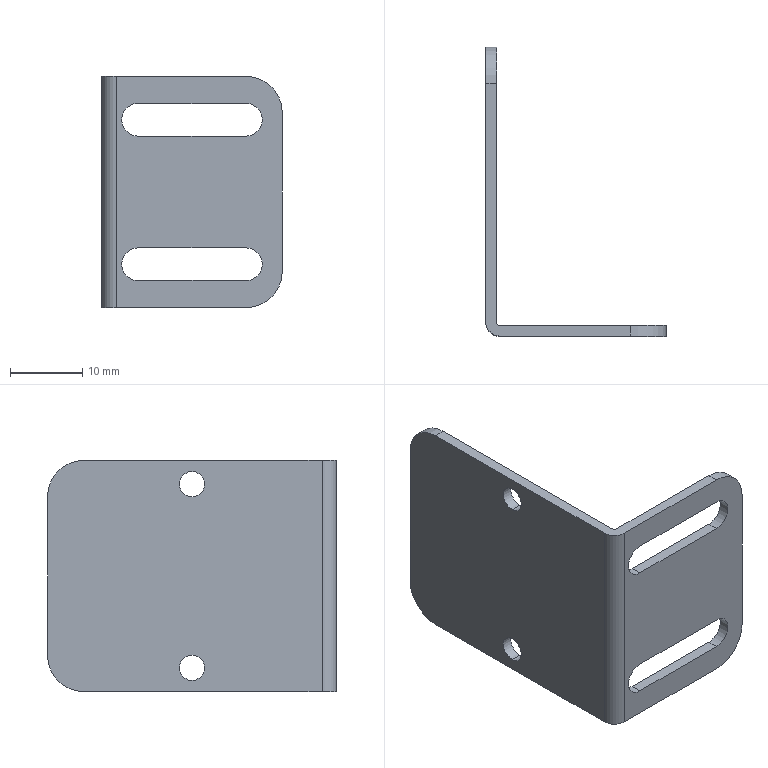Part | SolidWorks | features Fillet 3, ICE 2, ExtruThin 1 | 1 solid | 26 faces | box 25 x 40 x 32 mm | volume 2711 mm3 | cylinder 14 | plane 12 | commonest cylinder face diameters 3.5 x4 4.5 x4 10 x4 1 x1 4 x1
STEP:
#1=CARTESIAN_POINT('',(1.5,20.,26.95));
#2=VERTEX_POINT('',#1);
#3=CARTESIAN_POINT('',(1.5,20.,30.45));
#4=VERTEX_POINT('',#3);
#5=CARTESIAN_POINT('',(1.5,20.,28.7));
#6=DIRECTION('',(-1.,0.,0.));
#7=DIRECTION('',(0.,0.,-1.));
#8=AXIS2_PLACEMENT_3D('',#5,#6,#7);
#9=CIRCLE('',#8,1.75);
#10=EDGE_CURVE('',#2,#4,#9,.T.);
#11=ORIENTED_EDGE('',*,*,#10,.F.);
#12=CARTESIAN_POINT('',(0.,20.,26.95));
#13=VERTEX_POINT('',#12);
#14=CARTESIAN_POINT('',(25.001,20.,26.95));
#15=DIRECTION('',(-1.,0.,0.));
#16=VECTOR('',#15,1000.);
#17=LINE('',#14,#16);
#18=EDGE_CURVE('',#2,#13,#17,.T.);
#19=ORIENTED_EDGE('',*,*,#18,.T.);
#20=CARTESIAN_POINT('',(0.,20.,30.45));
#21=VERTEX_POINT('',#20);
#22=CARTESIAN_POINT('',(0.,20.,28.7));
#23=DIRECTION('',(-1.,0.,0.));
#24=DIRECTION('',(0.,0.,1.));
#25=AXIS2_PLACEMENT_3D('',#22,#23,#24);
#26=CIRCLE('',#25,1.75);
#27=EDGE_CURVE('',#13,#21,#26,.T.);
#28=ORIENTED_EDGE('',*,*,#27,.T.);
#29=CARTESIAN_POINT('',(25.001,20.,30.45));
#30=DIRECTION('',(-1.,0.,0.));
#31=VECTOR('',#30,1000.);
#32=LINE('',#29,#31);
#33=EDGE_CURVE('',#4,#21,#32,.T.);
#34=ORIENTED_EDGE('',*,*,#33,.F.);
#35=EDGE_LOOP('',(#11,#19,#28,#34));
#36=FACE_OUTER_BOUND('',#35,.T.);
#37=CARTESIAN_POINT('',(25.001,20.,28.7));
#38=DIRECTION('',(-1.,0.,0.));
#39=DIRECTION('',(0.,0.,1.));
#40=AXIS2_PLACEMENT_3D('',#37,#38,#39);
#41=CYLINDRICAL_SURFACE('',#40,1.75);
#42=ADVANCED_FACE('',(#36),#41,.F.);
#43=CARTESIAN_POINT('',(1.5,20.,1.55));
#44=VERTEX_POINT('',#43);
#45=CARTESIAN_POINT('',(1.5,20.,5.05));
#46=VERTEX_POINT('',#45);
#47=CARTESIAN_POINT('',(1.5,20.,3.3));
#48=DIRECTION('',(-1.,0.,0.));
#49=DIRECTION('',(0.,0.,-1.));
#50=AXIS2_PLACEMENT_3D('',#47,#48,#49);
#51=CIRCLE('',#50,1.75);
#52=EDGE_CURVE('',#44,#46,#51,.T.);
#53=ORIENTED_EDGE('',*,*,#52,.F.);
#54=CARTESIAN_POINT('',(0.,20.,1.55));
#55=VERTEX_POINT('',#54);
#56=CARTESIAN_POINT('',(25.001,20.,1.55));
#57=DIRECTION('',(-1.,0.,0.));
#58=VECTOR('',#57,1000.);
#59=LINE('',#56,#58);
#60=EDGE_CURVE('',#44,#55,#59,.T.);
#61=ORIENTED_EDGE('',*,*,#60,.T.);
#62=CARTESIAN_POINT('',(0.,20.,5.05));
#63=VERTEX_POINT('',#62);
#64=CARTESIAN_POINT('',(0.,20.,3.3));
#65=DIRECTION('',(-1.,0.,0.));
#66=DIRECTION('',(0.,0.,1.));
#67=AXIS2_PLACEMENT_3D('',#64,#65,#66);
#68=CIRCLE('',#67,1.75);
#69=EDGE_CURVE('',#55,#63,#68,.T.);
#70=ORIENTED_EDGE('',*,*,#69,.T.);
#71=CARTESIAN_POINT('',(25.001,20.,5.05));
#72=DIRECTION('',(-1.,0.,0.));
#73=VECTOR('',#72,1000.);
#74=LINE('',#71,#73);
#75=EDGE_CURVE('',#46,#63,#74,.T.);
#76=ORIENTED_EDGE('',*,*,#75,.F.);
#77=EDGE_LOOP('',(#53,#61,#70,#76));
#78=FACE_OUTER_BOUND('',#77,.T.);
#79=CARTESIAN_POINT('',(25.001,20.,3.3));
#80=DIRECTION('',(-1.,0.,0.));
#81=DIRECTION('',(0.,0.,1.));
#82=AXIS2_PLACEMENT_3D('',#79,#80,#81);
#83=CYLINDRICAL_SURFACE('',#82,1.75);
#84=ADVANCED_FACE('',(#78),#83,.F.);
#85=CARTESIAN_POINT('',(5.,0.,23.75));
#86=VERTEX_POINT('',#85);
#87=CARTESIAN_POINT('',(20.,0.,23.75));
#88=VERTEX_POINT('',#87);
#89=CARTESIAN_POINT('',(5.,0.,23.75));
#90=DIRECTION('',(1.,0.,0.));
#91=VECTOR('',#90,1000.);
#92=LINE('',#89,#91);
#93=EDGE_CURVE('',#86,#88,#92,.T.);
#94=ORIENTED_EDGE('',*,*,#93,.F.);
#95=CARTESIAN_POINT('',(5.,0.,28.25));
#96=VERTEX_POINT('',#95);
#97=CARTESIAN_POINT('',(5.,0.,26.));
#98=DIRECTION('',(0.,-1.,0.));
#99=DIRECTION('',(0.,0.,1.));
#100=AXIS2_PLACEMENT_3D('',#97,#98,#99);
#101=CIRCLE('',#100,2.25);
#102=EDGE_CURVE('',#96,#86,#101,.T.);
#103=ORIENTED_EDGE('',*,*,#102,.F.);
#104=CARTESIAN_POINT('',(20.,0.,28.25));
#105=VERTEX_POINT('',#104);
#106=CARTESIAN_POINT('',(5.,0.,28.25));
#107=DIRECTION('',(-1.,0.,0.));
#108=VECTOR('',#107,1000.);
#109=LINE('',#106,#108);
#110=EDGE_CURVE('',#105,#96,#109,.T.);
#111=ORIENTED_EDGE('',*,*,#110,.F.);
#112=CARTESIAN_POINT('',(20.,0.,26.));
#113=DIRECTION('',(0.,-1.,0.));
#114=DIRECTION('',(0.,0.,1.));
#115=AXIS2_PLACEMENT_3D('',#112,#113,#114);
#116=CIRCLE('',#115,2.25);
#117=EDGE_CURVE('',#88,#105,#116,.T.);
#118=ORIENTED_EDGE('',*,*,#117,.F.);
#119=EDGE_LOOP('',(#94,#103,#111,#118));
#120=FACE_BOUND('',#119,.T.);
#121=CARTESIAN_POINT('',(5.,0.,3.75));
#122=VERTEX_POINT('',#121);
#123=CARTESIAN_POINT('',(20.,0.,3.75));
#124=VERTEX_POINT('',#123);
#125=CARTESIAN_POINT('',(5.,0.,3.75));
#126=DIRECTION('',(1.,0.,0.));
#127=VECTOR('',#126,1000.);
#128=LINE('',#125,#127);
#129=EDGE_CURVE('',#122,#124,#128,.T.);
#130=ORIENTED_EDGE('',*,*,#129,.F.);
#131=CARTESIAN_POINT('',(5.,0.,8.25));
#132=VERTEX_POINT('',#131);
#133=CARTESIAN_POINT('',(5.,0.,6.));
#134=DIRECTION('',(0.,-1.,0.));
#135=DIRECTION('',(0.,0.,1.));
#136=AXIS2_PLACEMENT_3D('',#133,#134,#135);
#137=CIRCLE('',#136,2.25);
#138=EDGE_CURVE('',#132,#122,#137,.T.);
#139=ORIENTED_EDGE('',*,*,#138,.F.);
#140=CARTESIAN_POINT('',(20.,0.,8.25));
#141=VERTEX_POINT('',#140);
#142=CARTESIAN_POINT('',(5.,0.,8.25));
#143=DIRECTION('',(-1.,0.,0.));
#144=VECTOR('',#143,1000.);
#145=LINE('',#142,#144);
#146=EDGE_CURVE('',#141,#132,#145,.T.);
#147=ORIENTED_EDGE('',*,*,#146,.F.);
#148=CARTESIAN_POINT('',(20.,0.,6.));
#149=DIRECTION('',(0.,-1.,0.));
#150=DIRECTION('',(0.,0.,1.));
#151=AXIS2_PLACEMENT_3D('',#148,#149,#150);
#152=CIRCLE('',#151,2.25);
#153=EDGE_CURVE('',#124,#141,#152,.T.);
#154=ORIENTED_EDGE('',*,*,#153,.F.);
#155=EDGE_LOOP('',(#130,#139,#147,#154));
#156=FACE_BOUND('',#155,.T.);
#157=CARTESIAN_POINT('',(25.,0.,27.));
#158=VERTEX_POINT('',#157);
#159=CARTESIAN_POINT('',(25.,0.,5.));
#160=VERTEX_POINT('',#159);
#161=CARTESIAN_POINT('',(25.,0.,32.));
#162=DIRECTION('',(0.,0.,-1.));
#163=VECTOR('',#162,1000.);
#164=LINE('',#161,#163);
#165=EDGE_CURVE('',#158,#160,#164,.T.);
#166=ORIENTED_EDGE('',*,*,#165,.F.);
#167=CARTESIAN_POINT('',(20.,0.,32.));
#168=VERTEX_POINT('',#167);
#169=CARTESIAN_POINT('',(20.,0.,27.));
#170=DIRECTION('',(0.,-1.,0.));
#171=DIRECTION('',(0.,0.,1.));
#172=AXIS2_PLACEMENT_3D('',#169,#170,#171);
#173=CIRCLE('',#172,5.);
#174=EDGE_CURVE('',#158,#168,#173,.T.);
#175=ORIENTED_EDGE('',*,*,#174,.T.);
#176=CARTESIAN_POINT('',(2.,0.,32.));
#177=VERTEX_POINT('',#176);
#178=CARTESIAN_POINT('',(0.,0.,32.));
#179=DIRECTION('',(1.,0.,0.));
#180=VECTOR('',#179,1000.);
#181=LINE('',#178,#180);
#182=EDGE_CURVE('',#177,#168,#181,.T.);
#183=ORIENTED_EDGE('',*,*,#182,.F.);
#184=CARTESIAN_POINT('',(2.,0.,0.));
#185=VERTEX_POINT('',#184);
#186=CARTESIAN_POINT('',(2.,0.,32.));
#187=DIRECTION('',(0.,0.,-1.));
#188=VECTOR('',#187,1000.);
#189=LINE('',#186,#188);
#190=EDGE_CURVE('',#177,#185,#189,.T.);
#191=ORIENTED_EDGE('',*,*,#190,.T.);
#192=CARTESIAN_POINT('',(20.,0.,0.));
#193=VERTEX_POINT('',#192);
#194=CARTESIAN_POINT('',(0.,0.,0.));
#195=DIRECTION('',(1.,0.,0.));
#196=VECTOR('',#195,1000.);
#197=LINE('',#194,#196);
#198=EDGE_CURVE('',#185,#193,#197,.T.);
#199=ORIENTED_EDGE('',*,*,#198,.T.);
#200=CARTESIAN_POINT('',(20.,0.,5.));
#201=DIRECTION('',(0.,-1.,0.));
#202=DIRECTION('',(0.,0.,1.));
#203=AXIS2_PLACEMENT_3D('',#200,#201,#202);
#204=CIRCLE('',#203,5.);
#205=EDGE_CURVE('',#193,#160,#204,.T.);
#206=ORIENTED_EDGE('',*,*,#205,.T.);
#207=EDGE_LOOP('',(#166,#175,#183,#191,#199,#206));
#208=FACE_OUTER_BOUND('',#207,.T.);
#209=CARTESIAN_POINT('',(0.,0.,32.));
#210=DIRECTION('',(0.,1.,0.));
#211=DIRECTION('',(0.,0.,1.));
#212=AXIS2_PLACEMENT_3D('',#209,#210,#211);
#213=PLANE('',#212);
#214=ADVANCED_FACE('',(#120,#156,#208),#213,.F.);
#215=CARTESIAN_POINT('',(25.,1.5,27.));
#216=VERTEX_POINT('',#215);
#217=CARTESIAN_POINT('',(25.,1.5,5.));
#218=VERTEX_POINT('',#217);
#219=CARTESIAN_POINT('',(25.,1.5,32.));
#220=DIRECTION('',(0.,0.,-1.));
#221=VECTOR('',#220,1000.);
#222=LINE('',#219,#221);
#223=EDGE_CURVE('',#216,#218,#222,.T.);
#224=ORIENTED_EDGE('',*,*,#223,.F.);
#225=CARTESIAN_POINT('',(25.,0.,27.));
#226=DIRECTION('',(0.,-1.,0.));
#227=VECTOR('',#226,1000.);
#228=LINE('',#225,#227);
#229=EDGE_CURVE('',#216,#158,#228,.T.);
#230=ORIENTED_EDGE('',*,*,#229,.T.);
#231=ORIENTED_EDGE('',*,*,#165,.T.);
#232=CARTESIAN_POINT('',(25.,1.5,5.));
#233=DIRECTION('',(0.,1.,0.));
#234=VECTOR('',#233,1000.);
#235=LINE('',#232,#234);
#236=EDGE_CURVE('',#160,#218,#235,.T.);
#237=ORIENTED_EDGE('',*,*,#236,.T.);
#238=EDGE_LOOP('',(#224,#230,#231,#237));
#239=FACE_OUTER_BOUND('',#238,.T.);
#240=CARTESIAN_POINT('',(25.,1.5,32.));
#241=DIRECTION('',(1.,0.,0.));
#242=DIRECTION('',(0.,0.,-1.));
#243=AXIS2_PLACEMENT_3D('',#240,#241,#242);
#244=PLANE('',#243);
#245=ADVANCED_FACE('',(#239),#244,.T.);
#246=CARTESIAN_POINT('',(5.,1.5,23.75));
#247=VERTEX_POINT('',#246);
#248=CARTESIAN_POINT('',(5.,1.5,28.25));
#249=VERTEX_POINT('',#248);
#250=CARTESIAN_POINT('',(5.,1.5,26.));
#251=DIRECTION('',(0.,1.,0.));
#252=DIRECTION('',(0.,0.,1.));
#253=AXIS2_PLACEMENT_3D('',#250,#251,#252);
#254=CIRCLE('',#253,2.25);
#255=EDGE_CURVE('',#247,#249,#254,.T.);
#256=ORIENTED_EDGE('',*,*,#255,.F.);
#257=CARTESIAN_POINT('',(20.,1.5,23.75));
#258=VERTEX_POINT('',#257);
#259=CARTESIAN_POINT('',(5.,1.5,23.75));
#260=DIRECTION('',(-1.,0.,0.));
#261=VECTOR('',#260,1000.);
#262=LINE('',#259,#261);
#263=EDGE_CURVE('',#258,#247,#262,.T.);
#264=ORIENTED_EDGE('',*,*,#263,.F.);
#265=CARTESIAN_POINT('',(20.,1.5,28.25));
#266=VERTEX_POINT('',#265);
#267=CARTESIAN_POINT('',(20.,1.5,26.));
#268=DIRECTION('',(0.,1.,0.));
#269=DIRECTION('',(0.,0.,1.));
#270=AXIS2_PLACEMENT_3D('',#267,#268,#269);
#271=CIRCLE('',#270,2.25);
#272=EDGE_CURVE('',#266,#258,#271,.T.);
#273=ORIENTED_EDGE('',*,*,#272,.F.);
#274=CARTESIAN_POINT('',(5.,1.5,28.25));
#275=DIRECTION('',(1.,0.,0.));
#276=VECTOR('',#275,1000.);
#277=LINE('',#274,#276);
#278=EDGE_CURVE('',#249,#266,#277,.T.);
#279=ORIENTED_EDGE('',*,*,#278,.F.);
#280=EDGE_LOOP('',(#256,#264,#273,#279));
#281=FACE_BOUND('',#280,.T.);
#282=CARTESIAN_POINT('',(5.,1.5,3.75));
#283=VERTEX_POINT('',#282);
#284=CARTESIAN_POINT('',(5.,1.5,8.25));
#285=VERTEX_POINT('',#284);
#286=CARTESIAN_POINT('',(5.,1.5,6.));
#287=DIRECTION('',(0.,1.,0.));
#288=DIRECTION('',(0.,0.,1.));
#289=AXIS2_PLACEMENT_3D('',#286,#287,#288);
#290=CIRCLE('',#289,2.25);
#291=EDGE_CURVE('',#283,#285,#290,.T.);
#292=ORIENTED_EDGE('',*,*,#291,.F.);
#293=CARTESIAN_POINT('',(20.,1.5,3.75));
#294=VERTEX_POINT('',#293);
#295=CARTESIAN_POINT('',(5.,1.5,3.75));
#296=DIRECTION('',(-1.,0.,0.));
#297=VECTOR('',#296,1000.);
#298=LINE('',#295,#297);
#299=EDGE_CURVE('',#294,#283,#298,.T.);
#300=ORIENTED_EDGE('',*,*,#299,.F.);
#301=CARTESIAN_POINT('',(20.,1.5,8.25));
#302=VERTEX_POINT('',#301);
#303=CARTESIAN_POINT('',(20.,1.5,6.));
#304=DIRECTION('',(0.,1.,0.));
#305=DIRECTION('',(0.,0.,1.));
#306=AXIS2_PLACEMENT_3D('',#303,#304,#305);
#307=CIRCLE('',#306,2.25);
#308=EDGE_CURVE('',#302,#294,#307,.T.);
#309=ORIENTED_EDGE('',*,*,#308,.F.);
#310=CARTESIAN_POINT('',(5.,1.5,8.25));
#311=DIRECTION('',(1.,0.,0.));
#312=VECTOR('',#311,1000.);
#313=LINE('',#310,#312);
#314=EDGE_CURVE('',#285,#302,#313,.T.);
#315=ORIENTED_EDGE('',*,*,#314,.F.);
#316=EDGE_LOOP('',(#292,#300,#309,#315));
#317=FACE_BOUND('',#316,.T.);
#318=CARTESIAN_POINT('',(2.,1.5,32.));
#319=VERTEX_POINT('',#318);
#320=CARTESIAN_POINT('',(20.,1.5,32.));
#321=VERTEX_POINT('',#320);
#322=CARTESIAN_POINT('',(0.,1.5,32.));
#323=DIRECTION('',(1.,0.,0.));
#324=VECTOR('',#323,1000.);
#325=LINE('',#322,#324);
#326=EDGE_CURVE('',#319,#321,#325,.T.);
#327=ORIENTED_EDGE('',*,*,#326,.T.);
#328=CARTESIAN_POINT('',(20.,1.5,27.));
#329=DIRECTION('',(0.,1.,0.));
#330=DIRECTION('',(0.,0.,1.));
#331=AXIS2_PLACEMENT_3D('',#328,#329,#330);
#332=CIRCLE('',#331,5.);
#333=EDGE_CURVE('',#321,#216,#332,.T.);
#334=ORIENTED_EDGE('',*,*,#333,.T.);
#335=ORIENTED_EDGE('',*,*,#223,.T.);
#336=CARTESIAN_POINT('',(20.,1.5,0.));
#337=VERTEX_POINT('',#336);
#338=CARTESIAN_POINT('',(20.,1.5,5.));
#339=DIRECTION('',(0.,1.,0.));
#340=DIRECTION('',(0.,0.,1.));
#341=AXIS2_PLACEMENT_3D('',#338,#339,#340);
#342=CIRCLE('',#341,5.);
#343=EDGE_CURVE('',#218,#337,#342,.T.);
#344=ORIENTED_EDGE('',*,*,#343,.T.);
#345=CARTESIAN_POINT('',(2.,1.5,0.));
#346=VERTEX_POINT('',#345);
#347=CARTESIAN_POINT('',(0.,1.5,0.));
#348=DIRECTION('',(1.,0.,0.));
#349=VECTOR('',#348,1000.);
#350=LINE('',#347,#349);
#351=EDGE_CURVE('',#346,#337,#350,.T.);
#352=ORIENTED_EDGE('',*,*,#351,.F.);
#353=CARTESIAN_POINT('',(2.,1.5,32.));
#354=DIRECTION('',(0.,0.,1.));
#355=VECTOR('',#354,1000.);
#356=LINE('',#353,#355);
#357=EDGE_CURVE('',#346,#319,#356,.T.);
#358=ORIENTED_EDGE('',*,*,#357,.T.);
#359=EDGE_LOOP('',(#327,#334,#335,#344,#352,#358));
#360=FACE_OUTER_BOUND('',#359,.T.);
#361=CARTESIAN_POINT('',(0.,1.5,32.));
#362=DIRECTION('',(0.,1.,0.));
#363=DIRECTION('',(0.,0.,1.));
#364=AXIS2_PLACEMENT_3D('',#361,#362,#363);
#365=PLANE('',#364);
#366=ADVANCED_FACE('',(#281,#317,#360),#365,.T.);
#367=CARTESIAN_POINT('',(1.5,20.,28.7));
#368=DIRECTION('',(-1.,0.,0.));
#369=DIRECTION('',(0.,0.,-1.));
#370=AXIS2_PLACEMENT_3D('',#367,#368,#369);
#371=CIRCLE('',#370,1.75);
#372=EDGE_CURVE('',#4,#2,#371,.T.);
#373=ORIENTED_EDGE('',*,*,#372,.T.);
#374=ORIENTED_EDGE('',*,*,#10,.T.);
#375=EDGE_LOOP('',(#373,#374));
#376=FACE_BOUND('',#375,.T.);
#377=CARTESIAN_POINT('',(1.5,20.,3.3));
#378=DIRECTION('',(-1.,0.,0.));
#379=DIRECTION('',(0.,0.,-1.));
#380=AXIS2_PLACEMENT_3D('',#377,#378,#379);
#381=CIRCLE('',#380,1.75);
#382=EDGE_CURVE('',#46,#44,#381,.T.);
#383=ORIENTED_EDGE('',*,*,#382,.T.);
#384=ORIENTED_EDGE('',*,*,#52,.T.);
#385=EDGE_LOOP('',(#383,#384));
#386=FACE_BOUND('',#385,.T.);
#387=CARTESIAN_POINT('',(1.5,35.,0.));
#388=VERTEX_POINT('',#387);
#389=CARTESIAN_POINT('',(1.5,2.,0.));
#390=VERTEX_POINT('',#389);
#391=CARTESIAN_POINT('',(1.5,0.,0.));
#392=DIRECTION('',(0.,-1.,0.));
#393=VECTOR('',#392,1000.);
#394=LINE('',#391,#393);
#395=EDGE_CURVE('',#388,#390,#394,.T.);
#396=ORIENTED_EDGE('',*,*,#395,.F.);
#397=CARTESIAN_POINT('',(1.5,40.,5.));
#398=VERTEX_POINT('',#397);
#399=CARTESIAN_POINT('',(1.5,35.,5.));
#400=DIRECTION('',(1.,0.,0.));
#401=DIRECTION('',(0.,0.,-1.));
#402=AXIS2_PLACEMENT_3D('',#399,#400,#401);
#403=CIRCLE('',#402,5.);
#404=EDGE_CURVE('',#388,#398,#403,.T.);
#405=ORIENTED_EDGE('',*,*,#404,.T.);
#406=CARTESIAN_POINT('',(1.5,40.,27.));
#407=VERTEX_POINT('',#406);
#408=CARTESIAN_POINT('',(1.5,40.,32.));
#409=DIRECTION('',(0.,0.,-1.));
#410=VECTOR('',#409,1000.);
#411=LINE('',#408,#410);
#412=EDGE_CURVE('',#407,#398,#411,.T.);
#413=ORIENTED_EDGE('',*,*,#412,.F.);
#414=CARTESIAN_POINT('',(1.5,35.,32.));
#415=VERTEX_POINT('',#414);
#416=CARTESIAN_POINT('',(1.5,35.,27.));
#417=DIRECTION('',(1.,0.,0.));
#418=DIRECTION('',(0.,0.,-1.));
#419=AXIS2_PLACEMENT_3D('',#416,#417,#418);
#420=CIRCLE('',#419,5.);
#421=EDGE_CURVE('',#407,#415,#420,.T.);
#422=ORIENTED_EDGE('',*,*,#421,.T.);
#423=CARTESIAN_POINT('',(1.5,2.,32.));
#424=VERTEX_POINT('',#423);
#425=CARTESIAN_POINT('',(1.5,0.,32.));
#426=DIRECTION('',(0.,-1.,0.));
#427=VECTOR('',#426,1000.);
#428=LINE('',#425,#427);
#429=EDGE_CURVE('',#415,#424,#428,.T.);
#430=ORIENTED_EDGE('',*,*,#429,.T.);
#431=CARTESIAN_POINT('',(1.5,2.,0.));
#432=DIRECTION('',(0.,0.,-1.));
#433=VECTOR('',#432,1000.);
#434=LINE('',#431,#433);
#435=EDGE_CURVE('',#424,#390,#434,.T.);
#436=ORIENTED_EDGE('',*,*,#435,.T.);
#437=EDGE_LOOP('',(#396,#405,#413,#422,#430,#436));
#438=FACE_OUTER_BOUND('',#437,.T.);
#439=CARTESIAN_POINT('',(1.5,0.,32.));
#440=DIRECTION('',(1.,0.,0.));
#441=DIRECTION('',(0.,0.,-1.));
#442=AXIS2_PLACEMENT_3D('',#439,#440,#441);
#443=PLANE('',#442);
#444=ADVANCED_FACE('',(#376,#386,#438),#443,.T.);
#445=ORIENTED_EDGE('',*,*,#412,.T.);
#446=CARTESIAN_POINT('',(0.,40.,5.));
#447=VERTEX_POINT('',#446);
#448=CARTESIAN_POINT('',(0.,40.,5.));
#449=DIRECTION('',(-1.,0.,0.));
#450=VECTOR('',#449,1000.);
#451=LINE('',#448,#450);
#452=EDGE_CURVE('',#398,#447,#451,.T.);
#453=ORIENTED_EDGE('',*,*,#452,.T.);
#454=CARTESIAN_POINT('',(0.,40.,27.));
#455=VERTEX_POINT('',#454);
#456=CARTESIAN_POINT('',(0.,40.,32.));
#457=DIRECTION('',(0.,0.,-1.));
#458=VECTOR('',#457,1000.);
#459=LINE('',#456,#458);
#460=EDGE_CURVE('',#455,#447,#459,.T.);
#461=ORIENTED_EDGE('',*,*,#460,.F.);
#462=CARTESIAN_POINT('',(1.5,40.,27.));
#463=DIRECTION('',(1.,0.,0.));
#464=VECTOR('',#463,1000.);
#465=LINE('',#462,#464);
#466=EDGE_CURVE('',#455,#407,#465,.T.);
#467=ORIENTED_EDGE('',*,*,#466,.T.);
#468=EDGE_LOOP('',(#445,#453,#461,#467));
#469=FACE_OUTER_BOUND('',#468,.T.);
#470=CARTESIAN_POINT('',(0.,40.,32.));
#471=DIRECTION('',(0.,1.,0.));
#472=DIRECTION('',(0.,0.,1.));
#473=AXIS2_PLACEMENT_3D('',#470,#471,#472);
#474=PLANE('',#473);
#475=ADVANCED_FACE('',(#469),#474,.T.);
#476=CARTESIAN_POINT('',(0.,20.,28.7));
#477=DIRECTION('',(-1.,0.,0.));
#478=DIRECTION('',(0.,0.,1.));
#479=AXIS2_PLACEMENT_3D('',#476,#477,#478);
#480=CIRCLE('',#479,1.75);
#481=EDGE_CURVE('',#21,#13,#480,.T.);
#482=ORIENTED_EDGE('',*,*,#481,.F.);
#483=ORIENTED_EDGE('',*,*,#27,.F.);
#484=EDGE_LOOP('',(#482,#483));
#485=FACE_BOUND('',#484,.T.);
#486=CARTESIAN_POINT('',(0.,20.,3.3));
#487=DIRECTION('',(-1.,0.,0.));
#488=DIRECTION('',(0.,0.,1.));
#489=AXIS2_PLACEMENT_3D('',#486,#487,#488);
#490=CIRCLE('',#489,1.75);
#491=EDGE_CURVE('',#63,#55,#490,.T.);
#492=ORIENTED_EDGE('',*,*,#491,.F.);
#493=ORIENTED_EDGE('',*,*,#69,.F.);
#494=EDGE_LOOP('',(#492,#493));
#495=FACE_BOUND('',#494,.T.);
#496=ORIENTED_EDGE('',*,*,#460,.T.);
#497=CARTESIAN_POINT('',(0.,35.,0.));
#498=VERTEX_POINT('',#497);
#499=CARTESIAN_POINT('',(0.,35.,5.));
#500=DIRECTION('',(-1.,0.,0.));
#501=DIRECTION('',(0.,0.,-1.));
#502=AXIS2_PLACEMENT_3D('',#499,#500,#501);
#503=CIRCLE('',#502,5.);
#504=EDGE_CURVE('',#447,#498,#503,.T.);
#505=ORIENTED_EDGE('',*,*,#504,.T.);
#506=CARTESIAN_POINT('',(0.,2.,0.));
#507=VERTEX_POINT('',#506);
#508=CARTESIAN_POINT('',(0.,0.,0.));
#509=DIRECTION('',(0.,-1.,0.));
#510=VECTOR('',#509,1000.);
#511=LINE('',#508,#510);
#512=EDGE_CURVE('',#498,#507,#511,.T.);
#513=ORIENTED_EDGE('',*,*,#512,.T.);
#514=CARTESIAN_POINT('',(0.,2.,32.));
#515=VERTEX_POINT('',#514);
#516=CARTESIAN_POINT('',(0.,2.,32.));
#517=DIRECTION('',(0.,0.,1.));
#518=VECTOR('',#517,1000.);
#519=LINE('',#516,#518);
#520=EDGE_CURVE('',#507,#515,#519,.T.);
#521=ORIENTED_EDGE('',*,*,#520,.T.);
#522=CARTESIAN_POINT('',(0.,35.,32.));
#523=VERTEX_POINT('',#522);
#524=CARTESIAN_POINT('',(0.,0.,32.));
#525=DIRECTION('',(0.,-1.,0.));
#526=VECTOR('',#525,1000.);
#527=LINE('',#524,#526);
#528=EDGE_CURVE('',#523,#515,#527,.T.);
#529=ORIENTED_EDGE('',*,*,#528,.F.);
#530=CARTESIAN_POINT('',(0.,35.,27.));
#531=DIRECTION('',(-1.,0.,0.));
#532=DIRECTION('',(0.,0.,-1.));
#533=AXIS2_PLACEMENT_3D('',#530,#531,#532);
#534=CIRCLE('',#533,5.);
#535=EDGE_CURVE('',#523,#455,#534,.T.);
#536=ORIENTED_EDGE('',*,*,#535,.T.);
#537=EDGE_LOOP('',(#496,#505,#513,#521,#529,#536));
#538=FACE_OUTER_BOUND('',#537,.T.);
#539=CARTESIAN_POINT('',(0.,0.,32.));
#540=DIRECTION('',(1.,0.,0.));
#541=DIRECTION('',(0.,0.,-1.));
#542=AXIS2_PLACEMENT_3D('',#539,#540,#541);
#543=PLANE('',#542);
#544=ADVANCED_FACE('',(#485,#495,#538),#543,.F.);
#545=ORIENTED_EDGE('',*,*,#182,.T.);
#546=CARTESIAN_POINT('',(20.,1.5,32.));
#547=DIRECTION('',(0.,1.,0.));
#548=VECTOR('',#547,1000.);
#549=LINE('',#546,#548);
#550=EDGE_CURVE('',#168,#321,#549,.T.);
#551=ORIENTED_EDGE('',*,*,#550,.T.);
#552=ORIENTED_EDGE('',*,*,#326,.F.);
#553=CARTESIAN_POINT('',(2.,2.,32.));
#554=DIRECTION('',(0.,0.,-1.));
#555=DIRECTION('',(-1.,0.,0.));
#556=AXIS2_PLACEMENT_3D('',#553,#554,#555);
#557=CIRCLE('',#556,0.5);
#558=EDGE_CURVE('',#319,#424,#557,.T.);
#559=ORIENTED_EDGE('',*,*,#558,.T.);
#560=ORIENTED_EDGE('',*,*,#429,.F.);
#561=CARTESIAN_POINT('',(0.,35.,32.));
#562=DIRECTION('',(-1.,0.,0.));
#563=VECTOR('',#562,1000.);
#564=LINE('',#561,#563);
#565=EDGE_CURVE('',#415,#523,#564,.T.);
#566=ORIENTED_EDGE('',*,*,#565,.T.);
#567=ORIENTED_EDGE('',*,*,#528,.T.);
#568=CARTESIAN_POINT('',(2.,2.,32.));
#569=DIRECTION('',(0.,0.,1.));
#570=DIRECTION('',(-1.,0.,0.));
#571=AXIS2_PLACEMENT_3D('',#568,#569,#570);
#572=CIRCLE('',#571,2.);
#573=EDGE_CURVE('',#515,#177,#572,.T.);
#574=ORIENTED_EDGE('',*,*,#573,.T.);
#575=EDGE_LOOP('',(#545,#551,#552,#559,#560,#566,#567,#574));
#576=FACE_OUTER_BOUND('',#575,.T.);
#577=CARTESIAN_POINT('',(0.,0.,32.));
#578=DIRECTION('',(0.,0.,-1.));
#579=DIRECTION('',(-1.,0.,0.));
#580=AXIS2_PLACEMENT_3D('',#577,#578,#579);
#581=PLANE('',#580);
#582=ADVANCED_FACE('',(#576),#581,.F.);
#583=ORIENTED_EDGE('',*,*,#351,.T.);
#584=CARTESIAN_POINT('',(20.,0.,0.));
#585=DIRECTION('',(0.,-1.,0.));
#586=VECTOR('',#585,1000.);
#587=LINE('',#584,#586);
#588=EDGE_CURVE('',#337,#193,#587,.T.);
#589=ORIENTED_EDGE('',*,*,#588,.T.);
#590=ORIENTED_EDGE('',*,*,#198,.F.);
#591=CARTESIAN_POINT('',(2.,2.,0.));
#592=DIRECTION('',(0.,0.,-1.));
#593=DIRECTION('',(-1.,0.,0.));
#594=AXIS2_PLACEMENT_3D('',#591,#592,#593);
#595=CIRCLE('',#594,2.);
#596=EDGE_CURVE('',#185,#507,#595,.T.);
#597=ORIENTED_EDGE('',*,*,#596,.T.);
#598=ORIENTED_EDGE('',*,*,#512,.F.);
#599=CARTESIAN_POINT('',(0.,35.,0.));
#600=DIRECTION('',(1.,0.,0.));
#601=VECTOR('',#600,1000.);
#602=LINE('',#599,#601);
#603=EDGE_CURVE('',#498,#388,#602,.T.);
#604=ORIENTED_EDGE('',*,*,#603,.T.);
#605=ORIENTED_EDGE('',*,*,#395,.T.);
#606=CARTESIAN_POINT('',(2.,2.,0.));
#607=DIRECTION('',(0.,0.,1.));
#608=DIRECTION('',(-1.,0.,0.));
#609=AXIS2_PLACEMENT_3D('',#606,#607,#608);
#610=CIRCLE('',#609,0.5);
#611=EDGE_CURVE('',#390,#346,#610,.T.);
#612=ORIENTED_EDGE('',*,*,#611,.T.);
#613=EDGE_LOOP('',(#583,#589,#590,#597,#598,#604,#605,#612));
#614=FACE_OUTER_BOUND('',#613,.T.);
#615=CARTESIAN_POINT('',(0.,0.,0.));
#616=DIRECTION('',(0.,0.,-1.));
#617=DIRECTION('',(-1.,0.,0.));
#618=AXIS2_PLACEMENT_3D('',#615,#616,#617);
#619=PLANE('',#618);
#620=ADVANCED_FACE('',(#614),#619,.T.);
#621=ORIENTED_EDGE('',*,*,#558,.F.);
#622=ORIENTED_EDGE('',*,*,#357,.F.);
#623=ORIENTED_EDGE('',*,*,#611,.F.);
#624=ORIENTED_EDGE('',*,*,#435,.F.);
#625=EDGE_LOOP('',(#621,#622,#623,#624));
#626=FACE_OUTER_BOUND('',#625,.T.);
#627=CARTESIAN_POINT('',(2.,2.,32.));
#628=DIRECTION('',(0.,0.,1.));
#629=DIRECTION('',(1.,0.,0.));
#630=AXIS2_PLACEMENT_3D('',#627,#628,#629);
#631=CYLINDRICAL_SURFACE('',#630,0.5);
#632=ADVANCED_FACE('',(#626),#631,.F.);
#633=ORIENTED_EDGE('',*,*,#573,.F.);
#634=ORIENTED_EDGE('',*,*,#520,.F.);
#635=ORIENTED_EDGE('',*,*,#596,.F.);
#636=ORIENTED_EDGE('',*,*,#190,.F.);
#637=EDGE_LOOP('',(#633,#634,#635,#636));
#638=FACE_OUTER_BOUND('',#637,.T.);
#639=CARTESIAN_POINT('',(2.,2.,32.));
#640=DIRECTION('',(0.,0.,-1.));
#641=DIRECTION('',(-1.,0.,0.));
#642=AXIS2_PLACEMENT_3D('',#639,#640,#641);
#643=CYLINDRICAL_SURFACE('',#642,2.);
#644=ADVANCED_FACE('',(#638),#643,.T.);
#645=ORIENTED_EDGE('',*,*,#333,.F.);
#646=ORIENTED_EDGE('',*,*,#550,.F.);
#647=ORIENTED_EDGE('',*,*,#174,.F.);
#648=ORIENTED_EDGE('',*,*,#229,.F.);
#649=EDGE_LOOP('',(#645,#646,#647,#648));
#650=FACE_OUTER_BOUND('',#649,.T.);
#651=CARTESIAN_POINT('',(20.,1.5,27.));
#652=DIRECTION('',(0.,1.,0.));
#653=DIRECTION('',(0.,0.,1.));
#654=AXIS2_PLACEMENT_3D('',#651,#652,#653);
#655=CYLINDRICAL_SURFACE('',#654,5.);
#656=ADVANCED_FACE('',(#650),#655,.T.);
#657=ORIENTED_EDGE('',*,*,#343,.F.);
#658=ORIENTED_EDGE('',*,*,#236,.F.);
#659=ORIENTED_EDGE('',*,*,#205,.F.);
#660=ORIENTED_EDGE('',*,*,#588,.F.);
#661=EDGE_LOOP('',(#657,#658,#659,#660));
#662=FACE_OUTER_BOUND('',#661,.T.);
#663=CARTESIAN_POINT('',(20.,0.,5.));
#664=DIRECTION('',(0.,-1.,0.));
#665=DIRECTION('',(0.,0.,-1.));
#666=AXIS2_PLACEMENT_3D('',#663,#664,#665);
#667=CYLINDRICAL_SURFACE('',#666,5.);
#668=ADVANCED_FACE('',(#662),#667,.T.);
#669=ORIENTED_EDGE('',*,*,#504,.F.);
#670=ORIENTED_EDGE('',*,*,#452,.F.);
#671=ORIENTED_EDGE('',*,*,#404,.F.);
#672=ORIENTED_EDGE('',*,*,#603,.F.);
#673=EDGE_LOOP('',(#669,#670,#671,#672));
#674=FACE_OUTER_BOUND('',#673,.T.);
#675=CARTESIAN_POINT('',(0.,35.,5.));
#676=DIRECTION('',(1.,0.,0.));
#677=DIRECTION('',(0.,0.,-1.));
#678=AXIS2_PLACEMENT_3D('',#675,#676,#677);
#679=CYLINDRICAL_SURFACE('',#678,5.);
#680=ADVANCED_FACE('',(#674),#679,.T.);
#681=ORIENTED_EDGE('',*,*,#535,.F.);
#682=ORIENTED_EDGE('',*,*,#565,.F.);
#683=ORIENTED_EDGE('',*,*,#421,.F.);
#684=ORIENTED_EDGE('',*,*,#466,.F.);
#685=EDGE_LOOP('',(#681,#682,#683,#684));
#686=FACE_OUTER_BOUND('',#685,.T.);
#687=CARTESIAN_POINT('',(0.,35.,27.));
#688=DIRECTION('',(-1.,0.,0.));
#689=DIRECTION('',(0.,0.,1.));
#690=AXIS2_PLACEMENT_3D('',#687,#688,#689);
#691=CYLINDRICAL_SURFACE('',#690,5.);
#692=ADVANCED_FACE('',(#686),#691,.T.);
#693=ORIENTED_EDGE('',*,*,#60,.F.);
#694=ORIENTED_EDGE('',*,*,#382,.F.);
#695=ORIENTED_EDGE('',*,*,#75,.T.);
#696=ORIENTED_EDGE('',*,*,#491,.T.);
#697=EDGE_LOOP('',(#693,#694,#695,#696));
#698=FACE_OUTER_BOUND('',#697,.T.);
#699=CARTESIAN_POINT('',(25.001,20.,3.3));
#700=DIRECTION('',(-1.,0.,0.));
#701=DIRECTION('',(0.,0.,1.));
#702=AXIS2_PLACEMENT_3D('',#699,#700,#701);
#703=CYLINDRICAL_SURFACE('',#702,1.75);
#704=ADVANCED_FACE('',(#698),#703,.F.);
#705=ORIENTED_EDGE('',*,*,#18,.F.);
#706=ORIENTED_EDGE('',*,*,#372,.F.);
#707=ORIENTED_EDGE('',*,*,#33,.T.);
#708=ORIENTED_EDGE('',*,*,#481,.T.);
#709=EDGE_LOOP('',(#705,#706,#707,#708));
#710=FACE_OUTER_BOUND('',#709,.T.);
#711=CARTESIAN_POINT('',(25.001,20.,28.7));
#712=DIRECTION('',(-1.,0.,0.));
#713=DIRECTION('',(0.,0.,1.));
#714=AXIS2_PLACEMENT_3D('',#711,#712,#713);
#715=CYLINDRICAL_SURFACE('',#714,1.75);
#716=ADVANCED_FACE('',(#710),#715,.F.);
#717=ORIENTED_EDGE('',*,*,#138,.T.);
#718=CARTESIAN_POINT('',(5.,-0.001,3.75));
#719=DIRECTION('',(0.,1.,0.));
#720=VECTOR('',#719,1000.);
#721=LINE('',#718,#720);
#722=EDGE_CURVE('',#122,#283,#721,.T.);
#723=ORIENTED_EDGE('',*,*,#722,.T.);
#724=ORIENTED_EDGE('',*,*,#291,.T.);
#725=CARTESIAN_POINT('',(5.,-0.001,8.25));
#726=DIRECTION('',(0.,1.,0.));
#727=VECTOR('',#726,1000.);
#728=LINE('',#725,#727);
#729=EDGE_CURVE('',#132,#285,#728,.T.);
#730=ORIENTED_EDGE('',*,*,#729,.F.);
#731=EDGE_LOOP('',(#717,#723,#724,#730));
#732=FACE_OUTER_BOUND('',#731,.T.);
#733=CARTESIAN_POINT('',(5.,-0.001,6.));
#734=DIRECTION('',(0.,1.,0.));
#735=DIRECTION('',(0.,0.,1.));
#736=AXIS2_PLACEMENT_3D('',#733,#734,#735);
#737=CYLINDRICAL_SURFACE('',#736,2.25);
#738=ADVANCED_FACE('',(#732),#737,.F.);
#739=ORIENTED_EDGE('',*,*,#129,.T.);
#740=CARTESIAN_POINT('',(20.,-0.001,3.75));
#741=DIRECTION('',(0.,1.,0.));
#742=VECTOR('',#741,1000.);
#743=LINE('',#740,#742);
#744=EDGE_CURVE('',#124,#294,#743,.T.);
#745=ORIENTED_EDGE('',*,*,#744,.T.);
#746=ORIENTED_EDGE('',*,*,#299,.T.);
#747=ORIENTED_EDGE('',*,*,#722,.F.);
#748=EDGE_LOOP('',(#739,#745,#746,#747));
#749=FACE_OUTER_BOUND('',#748,.T.);
#750=CARTESIAN_POINT('',(5.,-0.001,3.75));
#751=DIRECTION('',(0.,0.,-1.));
#752=DIRECTION('',(-1.,0.,0.));
#753=AXIS2_PLACEMENT_3D('',#750,#751,#752);
#754=PLANE('',#753);
#755=ADVANCED_FACE('',(#749),#754,.F.);
#756=ORIENTED_EDGE('',*,*,#153,.T.);
#757=CARTESIAN_POINT('',(20.,-0.001,8.25));
#758=DIRECTION('',(0.,1.,0.));
#759=VECTOR('',#758,1000.);
#760=LINE('',#757,#759);
#761=EDGE_CURVE('',#141,#302,#760,.T.);
#762=ORIENTED_EDGE('',*,*,#761,.T.);
#763=ORIENTED_EDGE('',*,*,#308,.T.);
#764=ORIENTED_EDGE('',*,*,#744,.F.);
#765=EDGE_LOOP('',(#756,#762,#763,#764));
#766=FACE_OUTER_BOUND('',#765,.T.);
#767=CARTESIAN_POINT('',(20.,-0.001,6.));
#768=DIRECTION('',(0.,1.,0.));
#769=DIRECTION('',(0.,0.,1.));
#770=AXIS2_PLACEMENT_3D('',#767,#768,#769);
#771=CYLINDRICAL_SURFACE('',#770,2.25);
#772=ADVANCED_FACE('',(#766),#771,.F.);
#773=ORIENTED_EDGE('',*,*,#146,.T.);
#774=ORIENTED_EDGE('',*,*,#729,.T.);
#775=ORIENTED_EDGE('',*,*,#314,.T.);
#776=ORIENTED_EDGE('',*,*,#761,.F.);
#777=EDGE_LOOP('',(#773,#774,#775,#776));
#778=FACE_OUTER_BOUND('',#777,.T.);
#779=CARTESIAN_POINT('',(5.,-0.001,8.25));
#780=DIRECTION('',(0.,0.,1.));
#781=DIRECTION('',(1.,0.,0.));
#782=AXIS2_PLACEMENT_3D('',#779,#780,#781);
#783=PLANE('',#782);
#784=ADVANCED_FACE('',(#778),#783,.F.);
#785=ORIENTED_EDGE('',*,*,#102,.T.);
#786=CARTESIAN_POINT('',(5.,-0.001,23.75));
#787=DIRECTION('',(0.,1.,0.));
#788=VECTOR('',#787,1000.);
#789=LINE('',#786,#788);
#790=EDGE_CURVE('',#86,#247,#789,.T.);
#791=ORIENTED_EDGE('',*,*,#790,.T.);
#792=ORIENTED_EDGE('',*,*,#255,.T.);
#793=CARTESIAN_POINT('',(5.,-0.001,28.25));
#794=DIRECTION('',(0.,1.,0.));
#795=VECTOR('',#794,1000.);
#796=LINE('',#793,#795);
#797=EDGE_CURVE('',#96,#249,#796,.T.);
#798=ORIENTED_EDGE('',*,*,#797,.F.);
#799=EDGE_LOOP('',(#785,#791,#792,#798));
#800=FACE_OUTER_BOUND('',#799,.T.);
#801=CARTESIAN_POINT('',(5.,-0.001,26.));
#802=DIRECTION('',(0.,1.,0.));
#803=DIRECTION('',(0.,0.,1.));
#804=AXIS2_PLACEMENT_3D('',#801,#802,#803);
#805=CYLINDRICAL_SURFACE('',#804,2.25);
#806=ADVANCED_FACE('',(#800),#805,.F.);
#807=ORIENTED_EDGE('',*,*,#93,.T.);
#808=CARTESIAN_POINT('',(20.,-0.001,23.75));
#809=DIRECTION('',(0.,1.,0.));
#810=VECTOR('',#809,1000.);
#811=LINE('',#808,#810);
#812=EDGE_CURVE('',#88,#258,#811,.T.);
#813=ORIENTED_EDGE('',*,*,#812,.T.);
#814=ORIENTED_EDGE('',*,*,#263,.T.);
#815=ORIENTED_EDGE('',*,*,#790,.F.);
#816=EDGE_LOOP('',(#807,#813,#814,#815));
#817=FACE_OUTER_BOUND('',#816,.T.);
#818=CARTESIAN_POINT('',(5.,-0.001,23.75));
#819=DIRECTION('',(0.,0.,-1.));
#820=DIRECTION('',(-1.,0.,0.));
#821=AXIS2_PLACEMENT_3D('',#818,#819,#820);
#822=PLANE('',#821);
#823=ADVANCED_FACE('',(#817),#822,.F.);
#824=ORIENTED_EDGE('',*,*,#117,.T.);
#825=CARTESIAN_POINT('',(20.,-0.001,28.25));
#826=DIRECTION('',(0.,1.,0.));
#827=VECTOR('',#826,1000.);
#828=LINE('',#825,#827);
#829=EDGE_CURVE('',#105,#266,#828,.T.);
#830=ORIENTED_EDGE('',*,*,#829,.T.);
#831=ORIENTED_EDGE('',*,*,#272,.T.);
#832=ORIENTED_EDGE('',*,*,#812,.F.);
#833=EDGE_LOOP('',(#824,#830,#831,#832));
#834=FACE_OUTER_BOUND('',#833,.T.);
#835=CARTESIAN_POINT('',(20.,-0.001,26.));
#836=DIRECTION('',(0.,1.,0.));
#837=DIRECTION('',(0.,0.,1.));
#838=AXIS2_PLACEMENT_3D('',#835,#836,#837);
#839=CYLINDRICAL_SURFACE('',#838,2.25);
#840=ADVANCED_FACE('',(#834),#839,.F.);
#841=ORIENTED_EDGE('',*,*,#110,.T.);
#842=ORIENTED_EDGE('',*,*,#797,.T.);
#843=ORIENTED_EDGE('',*,*,#278,.T.);
#844=ORIENTED_EDGE('',*,*,#829,.F.);
#845=EDGE_LOOP('',(#841,#842,#843,#844));
#846=FACE_OUTER_BOUND('',#845,.T.);
#847=CARTESIAN_POINT('',(5.,-0.001,28.25));
#848=DIRECTION('',(0.,0.,1.));
#849=DIRECTION('',(1.,0.,0.));
#850=AXIS2_PLACEMENT_3D('',#847,#848,#849);
#851=PLANE('',#850);
#852=ADVANCED_FACE('',(#846),#851,.F.);
#853=CLOSED_SHELL('',(#42,#84,#214,#245,#366,#444,#475,#544,#582,#620,#632,#644,#656,#668,#680,#692,#704,#716,#738,#755,#772,#784,#806,#823,#840,#852));
#854=MANIFOLD_SOLID_BREP('',#853);
#855=CARTESIAN_POINT('',(0.,0.,0.));
#856=DIRECTION('',(0.,0.,1.));
#857=DIRECTION('',(1.,0.,0.));
#858=AXIS2_PLACEMENT_3D('',#855,#856,#857);
#859=(LENGTH_UNIT()NAMED_UNIT(*)SI_UNIT(.MILLI.,.METRE.));
#860=UNCERTAINTY_MEASURE_WITH_UNIT(LENGTH_MEASURE(0.00001),#859,'','');
#861=(NAMED_UNIT(*)PLANE_ANGLE_UNIT()SI_UNIT($,.RADIAN.));
#862=(NAMED_UNIT(*)SI_UNIT($,.STERADIAN.)SOLID_ANGLE_UNIT());
#863=(GEOMETRIC_REPRESENTATION_CONTEXT(3)GLOBAL_UNCERTAINTY_ASSIGNED_CONTEXT((#860))GLOBAL_UNIT_ASSIGNED_CONTEXT((#859,#861,#862))REPRESENTATION_CONTEXT('',''));
#864=ADVANCED_BREP_SHAPE_REPRESENTATION('',(#854,#858),#863);